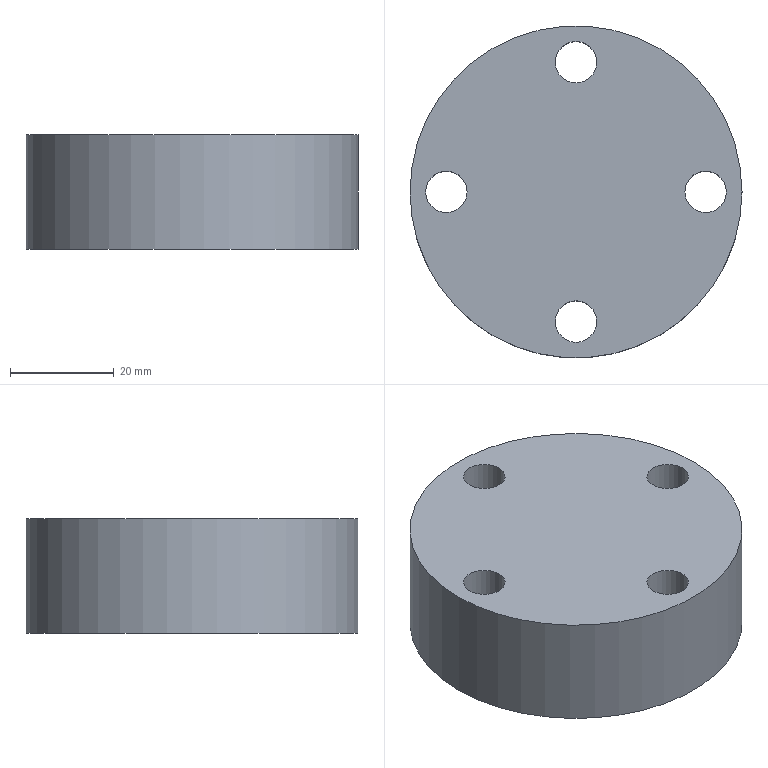NC program | NX | posted with a generic post | part box 64 x 64 x 22 mm
Whole program:
N10 G17 G21 G94 G90
(DRILLING , TOOL : ZXZ)
N12 T01 M6
N14 G54
N16 G17 G0 G90 X25. Y0. S3000 M3
N18 G43 Z30. H1
N20 G94 G81 G98 Z-1. F200. R3.
N22 X0. Y25.
N24 Y-25.
N26 X-25. Y0.
N28 G80
N30 G0 X-25. Y0. Z30.
N32 M5
(DRILLING_COPY , TOOL : 8.0ZT)
N34 T03 M6
N36 G54
N38 G17 G0 G90 X25. Y0. S1200 M3
N40 G43 Z30. H3
N42 G94 G83 G98 Z-25.903 F150. Q2. R3.
N44 X0. Y25.
N46 Y-25.
N48 X-25. Y0.
N50 G80
N52 G0 X-25. Y0. Z30.
N54 M5
(ZLEVEL_PROFILE_1_COPY_1 , TOOL : D6A45)
N56 T07 M6
N58 G54
N60 G17 G0 G90 X-26.351 Y1.37 S7500 M3
N62 G43 Z30. H7
N64 Z0.
N66 G94 G1 Z-1. F1000.
N68 X-27.824 Y0.52
N70 G3 X-28.124 Y0. R0.6
N72 X-25. Y-3.124 R3.124
N74 X-28.124 Y0. R-3.124
N76 X-27.824 Y-0.52 R0.6
N78 G1 X-26.351 Y-1.37
N80 Z0.
N82 G0 Z30.
N84 X1.37 Y26.351
N86 Z0.
N88 G1 Z-1.
N90 X0.52 Y27.824
N92 G3 X0. Y28.124 R0.6
N94 X-3.124 Y25. R3.124
N96 X0. Y28.124 R-3.124
N98 X-0.52 Y27.824 R0.6
N100 G1 X-1.37 Y26.351
N102 Z0.
N104 G0 Z30.
N106 X26.351 Y-1.37
N108 Z0.
N110 G1 Z-1.
N112 X27.824 Y-0.52
N114 G3 X28.124 Y0. R0.6
N116 X25. Y3.124 R3.124
N118 X28.124 Y0. R-3.124
N120 X27.824 Y0.52 R0.6
N122 G1 X26.351 Y1.37
N124 Z0.
N126 G0 Z30.
N128 X-1.37 Y-26.351
N130 Z0.
N132 G1 Z-1.
N134 X-0.52 Y-27.824
N136 G3 X0. Y-28.124 R0.6
N138 X3.124 Y-25. R3.124
N140 X0. Y-28.124 R-3.124
N142 X0.52 Y-27.824 R0.6
N144 G1 X1.37 Y-26.351
N146 Z0.
N148 G0 Z30.
N150 M5
N152 M2